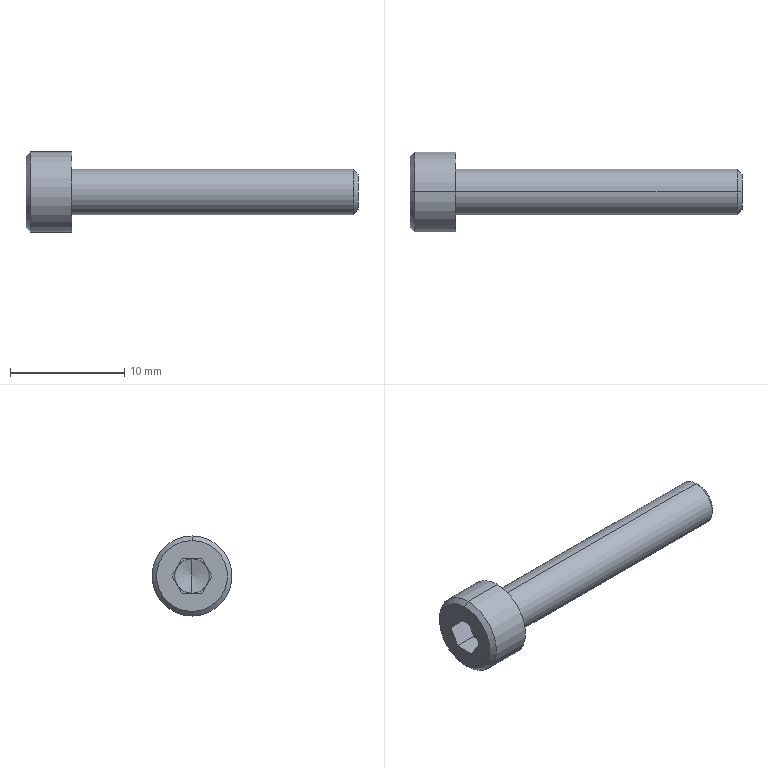Part | STEP file | 0246_306_SCB4-25 | 1 solid | 25 faces | box 29 x 7 x 7 mm | volume 448.793 mm3 | plane 15 | cone 6 | cylinder 4 | commonest cylinder face diameters 4 x2 7 x2